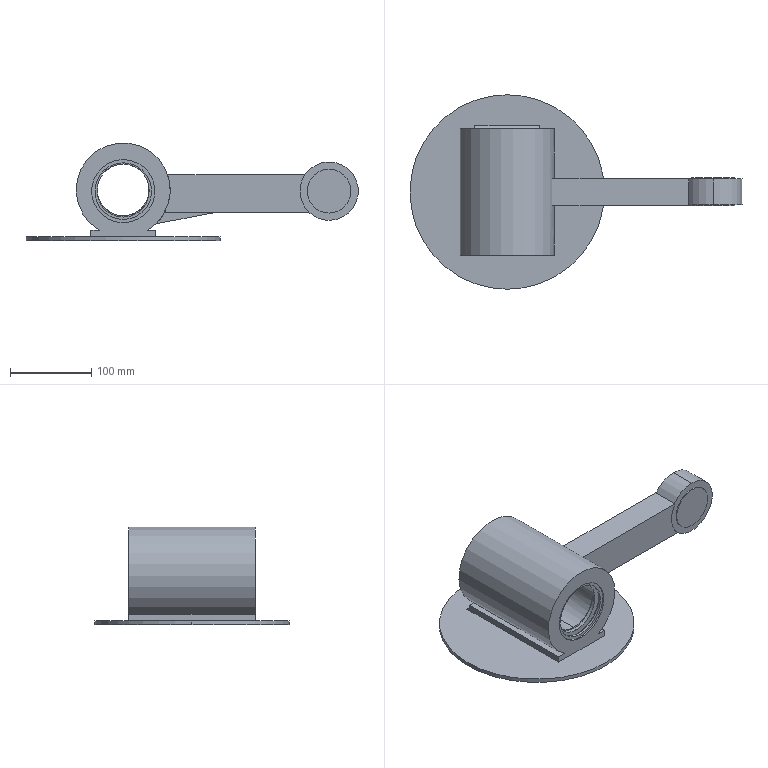Part | STEP file | Axle box 1 | 1 solid | 50 faces | box 410 x 240 x 120.8 mm | volume 1300329 mm3 | cylinder 25 | plane 25 | commonest cylinder face diameters 72 x5 54 x4 64 x4 70 x2 78 x2 78.4 x2
STEP:
#1=CARTESIAN_POINT('',(0.,-16.,-27.));
#2=VERTEX_POINT('',#1);
#3=CARTESIAN_POINT('',(0.,-16.,27.));
#4=VERTEX_POINT('',#3);
#5=CARTESIAN_POINT('',(0.,-16.,0.));
#6=DIRECTION('',(0.,-1.,0.));
#7=DIRECTION('',(0.,0.,1.));
#8=AXIS2_PLACEMENT_3D('',#5,#6,#7);
#9=CIRCLE('',#8,27.);
#10=EDGE_CURVE('',#2,#4,#9,.T.);
#11=ORIENTED_EDGE('',*,*,#10,.T.);
#12=CARTESIAN_POINT('',(0.,-17.2,27.));
#13=VERTEX_POINT('',#12);
#14=CARTESIAN_POINT('',(0.,17.2,27.));
#15=DIRECTION('',(0.,-1.,0.));
#16=VECTOR('',#15,1000.);
#17=LINE('',#14,#16);
#18=EDGE_CURVE('',#4,#13,#17,.T.);
#19=ORIENTED_EDGE('',*,*,#18,.T.);
#20=CARTESIAN_POINT('',(0.,-17.2,-27.));
#21=VERTEX_POINT('',#20);
#22=CARTESIAN_POINT('',(0.,-17.2,0.));
#23=DIRECTION('',(0.,1.,0.));
#24=DIRECTION('',(0.,0.,1.));
#25=AXIS2_PLACEMENT_3D('',#22,#23,#24);
#26=CIRCLE('',#25,27.);
#27=EDGE_CURVE('',#13,#21,#26,.T.);
#28=ORIENTED_EDGE('',*,*,#27,.T.);
#29=CARTESIAN_POINT('',(0.,17.2,-27.));
#30=DIRECTION('',(0.,-1.,0.));
#31=VECTOR('',#30,1000.);
#32=LINE('',#29,#31);
#33=EDGE_CURVE('',#2,#21,#32,.T.);
#34=ORIENTED_EDGE('',*,*,#33,.F.);
#35=EDGE_LOOP('',(#11,#19,#28,#34));
#36=FACE_OUTER_BOUND('',#35,.T.);
#37=CARTESIAN_POINT('',(0.,17.2,0.));
#38=DIRECTION('',(0.,-1.,0.));
#39=DIRECTION('',(0.,0.,-1.));
#40=AXIS2_PLACEMENT_3D('',#37,#38,#39);
#41=CYLINDRICAL_SURFACE('',#40,27.);
#42=ADVANCED_FACE('',(#36),#41,.T.);
#43=CARTESIAN_POINT('',(0.,17.2,27.));
#44=VERTEX_POINT('',#43);
#45=CARTESIAN_POINT('',(0.,17.2,-27.));
#46=VERTEX_POINT('',#45);
#47=CARTESIAN_POINT('',(0.,17.2,0.));
#48=DIRECTION('',(0.,1.,0.));
#49=DIRECTION('',(0.,0.,1.));
#50=AXIS2_PLACEMENT_3D('',#47,#48,#49);
#51=CIRCLE('',#50,27.);
#52=EDGE_CURVE('',#44,#46,#51,.T.);
#53=ORIENTED_EDGE('',*,*,#52,.F.);
#54=CARTESIAN_POINT('',(0.,16.,27.));
#55=VERTEX_POINT('',#54);
#56=CARTESIAN_POINT('',(0.,17.2,27.));
#57=DIRECTION('',(0.,-1.,0.));
#58=VECTOR('',#57,1000.);
#59=LINE('',#56,#58);
#60=EDGE_CURVE('',#44,#55,#59,.T.);
#61=ORIENTED_EDGE('',*,*,#60,.T.);
#62=CARTESIAN_POINT('',(0.,16.,-27.));
#63=VERTEX_POINT('',#62);
#64=CARTESIAN_POINT('',(0.,16.,0.));
#65=DIRECTION('',(0.,1.,0.));
#66=DIRECTION('',(0.,0.,1.));
#67=AXIS2_PLACEMENT_3D('',#64,#65,#66);
#68=CIRCLE('',#67,27.);
#69=EDGE_CURVE('',#55,#63,#68,.T.);
#70=ORIENTED_EDGE('',*,*,#69,.T.);
#71=CARTESIAN_POINT('',(0.,17.2,-27.));
#72=DIRECTION('',(0.,-1.,0.));
#73=VECTOR('',#72,1000.);
#74=LINE('',#71,#73);
#75=EDGE_CURVE('',#46,#63,#74,.T.);
#76=ORIENTED_EDGE('',*,*,#75,.F.);
#77=EDGE_LOOP('',(#53,#61,#70,#76));
#78=FACE_OUTER_BOUND('',#77,.T.);
#79=CARTESIAN_POINT('',(0.,17.2,0.));
#80=DIRECTION('',(0.,-1.,0.));
#81=DIRECTION('',(0.,0.,-1.));
#82=AXIS2_PLACEMENT_3D('',#79,#80,#81);
#83=CYLINDRICAL_SURFACE('',#82,27.);
#84=ADVANCED_FACE('',(#78),#83,.T.);
#85=CARTESIAN_POINT('',(-254.,-69.04,39.2));
#86=VERTEX_POINT('',#85);
#87=CARTESIAN_POINT('',(-254.,-69.04,-39.2));
#88=VERTEX_POINT('',#87);
#89=CARTESIAN_POINT('',(-254.,-69.04,0.));
#90=DIRECTION('',(0.,-1.,0.));
#91=DIRECTION('',(0.,0.,-1.));
#92=AXIS2_PLACEMENT_3D('',#89,#90,#91);
#93=CIRCLE('',#92,39.2);
#94=EDGE_CURVE('',#86,#88,#93,.T.);
#95=ORIENTED_EDGE('',*,*,#94,.F.);
#96=CARTESIAN_POINT('',(-254.,-73.04,39.2));
#97=VERTEX_POINT('',#96);
#98=CARTESIAN_POINT('',(-254.,-78.,39.2));
#99=DIRECTION('',(0.,-1.,0.));
#100=VECTOR('',#99,1000.);
#101=LINE('',#98,#100);
#102=EDGE_CURVE('',#86,#97,#101,.T.);
#103=ORIENTED_EDGE('',*,*,#102,.T.);
#104=CARTESIAN_POINT('',(-254.,-73.04,-39.2));
#105=VERTEX_POINT('',#104);
#106=CARTESIAN_POINT('',(-254.,-73.04,0.));
#107=DIRECTION('',(0.,-1.,0.));
#108=DIRECTION('',(0.,0.,-1.));
#109=AXIS2_PLACEMENT_3D('',#106,#107,#108);
#110=CIRCLE('',#109,39.2);
#111=EDGE_CURVE('',#97,#105,#110,.T.);
#112=ORIENTED_EDGE('',*,*,#111,.T.);
#113=CARTESIAN_POINT('',(-254.,-78.,-39.2));
#114=DIRECTION('',(0.,-1.,0.));
#115=VECTOR('',#114,1000.);
#116=LINE('',#113,#115);
#117=EDGE_CURVE('',#88,#105,#116,.T.);
#118=ORIENTED_EDGE('',*,*,#117,.F.);
#119=EDGE_LOOP('',(#95,#103,#112,#118));
#120=FACE_OUTER_BOUND('',#119,.T.);
#121=CARTESIAN_POINT('',(-254.,-78.,0.));
#122=DIRECTION('',(0.,-1.,0.));
#123=DIRECTION('',(0.,0.,-1.));
#124=AXIS2_PLACEMENT_3D('',#121,#122,#123);
#125=CYLINDRICAL_SURFACE('',#124,39.2);
#126=ADVANCED_FACE('',(#120),#125,.F.);
#127=CARTESIAN_POINT('',(-254.,-73.04,35.));
#128=VERTEX_POINT('',#127);
#129=CARTESIAN_POINT('',(-254.,-73.04,-35.));
#130=VERTEX_POINT('',#129);
#131=CARTESIAN_POINT('',(-254.,-73.04,0.));
#132=DIRECTION('',(0.,-1.,0.));
#133=DIRECTION('',(0.,0.,-1.));
#134=AXIS2_PLACEMENT_3D('',#131,#132,#133);
#135=CIRCLE('',#134,35.);
#136=EDGE_CURVE('',#128,#130,#135,.T.);
#137=ORIENTED_EDGE('',*,*,#136,.F.);
#138=CARTESIAN_POINT('',(-254.,-75.92,35.));
#139=VERTEX_POINT('',#138);
#140=CARTESIAN_POINT('',(-254.,-78.,35.));
#141=DIRECTION('',(0.,-1.,0.));
#142=VECTOR('',#141,1000.);
#143=LINE('',#140,#142);
#144=EDGE_CURVE('',#128,#139,#143,.T.);
#145=ORIENTED_EDGE('',*,*,#144,.T.);
#146=CARTESIAN_POINT('',(-254.,-75.92,-35.));
#147=VERTEX_POINT('',#146);
#148=CARTESIAN_POINT('',(-254.,-75.92,0.));
#149=DIRECTION('',(0.,-1.,0.));
#150=DIRECTION('',(0.,0.,-1.));
#151=AXIS2_PLACEMENT_3D('',#148,#149,#150);
#152=CIRCLE('',#151,35.);
#153=EDGE_CURVE('',#139,#147,#152,.T.);
#154=ORIENTED_EDGE('',*,*,#153,.T.);
#155=CARTESIAN_POINT('',(-254.,-78.,-35.));
#156=DIRECTION('',(0.,-1.,0.));
#157=VECTOR('',#156,1000.);
#158=LINE('',#155,#157);
#159=EDGE_CURVE('',#130,#147,#158,.T.);
#160=ORIENTED_EDGE('',*,*,#159,.F.);
#161=EDGE_LOOP('',(#137,#145,#154,#160));
#162=FACE_OUTER_BOUND('',#161,.T.);
#163=CARTESIAN_POINT('',(-254.,-78.,0.));
#164=DIRECTION('',(0.,-1.,0.));
#165=DIRECTION('',(0.,0.,-1.));
#166=AXIS2_PLACEMENT_3D('',#163,#164,#165);
#167=CYLINDRICAL_SURFACE('',#166,35.);
#168=ADVANCED_FACE('',(#162),#167,.F.);
#169=CARTESIAN_POINT('',(-254.,-75.92,39.));
#170=VERTEX_POINT('',#169);
#171=CARTESIAN_POINT('',(-254.,-75.92,-39.));
#172=VERTEX_POINT('',#171);
#173=CARTESIAN_POINT('',(-254.,-75.92,0.));
#174=DIRECTION('',(0.,-1.,0.));
#175=DIRECTION('',(0.,0.,-1.));
#176=AXIS2_PLACEMENT_3D('',#173,#174,#175);
#177=CIRCLE('',#176,39.);
#178=EDGE_CURVE('',#170,#172,#177,.T.);
#179=ORIENTED_EDGE('',*,*,#178,.F.);
#180=CARTESIAN_POINT('',(-254.,-78.,39.));
#181=VERTEX_POINT('',#180);
#182=CARTESIAN_POINT('',(-254.,-78.,39.));
#183=DIRECTION('',(0.,-1.,0.));
#184=VECTOR('',#183,1000.);
#185=LINE('',#182,#184);
#186=EDGE_CURVE('',#170,#181,#185,.T.);
#187=ORIENTED_EDGE('',*,*,#186,.T.);
#188=CARTESIAN_POINT('',(-254.,-78.,-39.));
#189=VERTEX_POINT('',#188);
#190=CARTESIAN_POINT('',(-254.,-78.,0.));
#191=DIRECTION('',(0.,-1.,0.));
#192=DIRECTION('',(0.,0.,-1.));
#193=AXIS2_PLACEMENT_3D('',#190,#191,#192);
#194=CIRCLE('',#193,39.);
#195=EDGE_CURVE('',#181,#189,#194,.T.);
#196=ORIENTED_EDGE('',*,*,#195,.T.);
#197=CARTESIAN_POINT('',(-254.,-78.,-39.));
#198=DIRECTION('',(0.,-1.,0.));
#199=VECTOR('',#198,1000.);
#200=LINE('',#197,#199);
#201=EDGE_CURVE('',#172,#189,#200,.T.);
#202=ORIENTED_EDGE('',*,*,#201,.F.);
#203=EDGE_LOOP('',(#179,#187,#196,#202));
#204=FACE_OUTER_BOUND('',#203,.T.);
#205=CARTESIAN_POINT('',(-254.,-78.,0.));
#206=DIRECTION('',(0.,-1.,0.));
#207=DIRECTION('',(0.,0.,-1.));
#208=AXIS2_PLACEMENT_3D('',#205,#206,#207);
#209=CYLINDRICAL_SURFACE('',#208,39.);
#210=ADVANCED_FACE('',(#204),#209,.F.);
#211=CARTESIAN_POINT('',(-254.,-64.8,-32.));
#212=VERTEX_POINT('',#211);
#213=CARTESIAN_POINT('',(-222.01,-64.8,0.8));
#214=VERTEX_POINT('',#213);
#215=CARTESIAN_POINT('',(-254.,-64.8,0.));
#216=DIRECTION('',(0.,-1.,0.));
#217=DIRECTION('',(0.,0.,-1.));
#218=AXIS2_PLACEMENT_3D('',#215,#216,#217);
#219=CIRCLE('',#218,32.);
#220=EDGE_CURVE('',#212,#214,#219,.T.);
#221=ORIENTED_EDGE('',*,*,#220,.F.);
#222=CARTESIAN_POINT('',(-254.,-69.04,-32.));
#223=VERTEX_POINT('',#222);
#224=CARTESIAN_POINT('',(-254.,-78.,-32.));
#225=DIRECTION('',(0.,-1.,0.));
#226=VECTOR('',#225,1000.);
#227=LINE('',#224,#226);
#228=EDGE_CURVE('',#212,#223,#227,.T.);
#229=ORIENTED_EDGE('',*,*,#228,.T.);
#230=CARTESIAN_POINT('',(-222.01,-69.04,0.8));
#231=VERTEX_POINT('',#230);
#232=CARTESIAN_POINT('',(-254.,-69.04,0.));
#233=DIRECTION('',(0.,-1.,0.));
#234=DIRECTION('',(0.,0.,-1.));
#235=AXIS2_PLACEMENT_3D('',#232,#233,#234);
#236=CIRCLE('',#235,32.);
#237=EDGE_CURVE('',#223,#231,#236,.T.);
#238=ORIENTED_EDGE('',*,*,#237,.T.);
#239=CARTESIAN_POINT('',(-222.01,-66.92,0.8));
#240=DIRECTION('',(0.,-1.,0.));
#241=VECTOR('',#240,1000.);
#242=LINE('',#239,#241);
#243=EDGE_CURVE('',#214,#231,#242,.T.);
#244=ORIENTED_EDGE('',*,*,#243,.F.);
#245=EDGE_LOOP('',(#221,#229,#238,#244));
#246=FACE_OUTER_BOUND('',#245,.T.);
#247=CARTESIAN_POINT('',(-254.,-78.,0.));
#248=DIRECTION('',(0.,-1.,0.));
#249=DIRECTION('',(0.,0.,-1.));
#250=AXIS2_PLACEMENT_3D('',#247,#248,#249);
#251=CYLINDRICAL_SURFACE('',#250,32.);
#252=ADVANCED_FACE('',(#246),#251,.F.);
#253=CARTESIAN_POINT('',(-374.,0.,-61.2));
#254=VERTEX_POINT('',#253);
#255=CARTESIAN_POINT('',(-134.,0.,-61.2));
#256=VERTEX_POINT('',#255);
#257=CARTESIAN_POINT('',(-254.,0.,-61.2));
#258=DIRECTION('',(0.,0.,-1.));
#259=DIRECTION('',(-1.,0.,0.));
#260=AXIS2_PLACEMENT_3D('',#257,#258,#259);
#261=CIRCLE('',#260,120.);
#262=EDGE_CURVE('',#254,#256,#261,.T.);
#263=ORIENTED_EDGE('',*,*,#262,.F.);
#264=CARTESIAN_POINT('',(-374.,0.,-56.4));
#265=VERTEX_POINT('',#264);
#266=CARTESIAN_POINT('',(-374.,0.,-61.2));
#267=DIRECTION('',(0.,0.,1.));
#268=VECTOR('',#267,1000.);
#269=LINE('',#266,#268);
#270=EDGE_CURVE('',#254,#265,#269,.T.);
#271=ORIENTED_EDGE('',*,*,#270,.T.);
#272=CARTESIAN_POINT('',(-134.,0.,-56.4));
#273=VERTEX_POINT('',#272);
#274=CARTESIAN_POINT('',(-254.,0.,-56.4));
#275=DIRECTION('',(0.,0.,-1.));
#276=DIRECTION('',(-1.,0.,0.));
#277=AXIS2_PLACEMENT_3D('',#274,#275,#276);
#278=CIRCLE('',#277,120.);
#279=EDGE_CURVE('',#265,#273,#278,.T.);
#280=ORIENTED_EDGE('',*,*,#279,.T.);
#281=CARTESIAN_POINT('',(-134.,0.,-61.2));
#282=DIRECTION('',(0.,0.,1.));
#283=VECTOR('',#282,1000.);
#284=LINE('',#281,#283);
#285=EDGE_CURVE('',#256,#273,#284,.T.);
#286=ORIENTED_EDGE('',*,*,#285,.F.);
#287=EDGE_LOOP('',(#263,#271,#280,#286));
#288=FACE_OUTER_BOUND('',#287,.T.);
#289=CARTESIAN_POINT('',(-254.,0.,-61.2));
#290=DIRECTION('',(0.,0.,1.));
#291=DIRECTION('',(1.,0.,0.));
#292=AXIS2_PLACEMENT_3D('',#289,#290,#291);
#293=CYLINDRICAL_SURFACE('',#292,120.);
#294=ADVANCED_FACE('',(#288),#293,.T.);
#295=CARTESIAN_POINT('',(-285.99,-64.8,0.8));
#296=VERTEX_POINT('',#295);
#297=CARTESIAN_POINT('',(-254.,-64.8,-30.4));
#298=VERTEX_POINT('',#297);
#299=CARTESIAN_POINT('',(-254.,-64.8,1.6));
#300=DIRECTION('',(0.,-1.,0.));
#301=DIRECTION('',(0.,0.,1.));
#302=AXIS2_PLACEMENT_3D('',#299,#300,#301);
#303=CIRCLE('',#302,32.);
#304=EDGE_CURVE('',#296,#298,#303,.T.);
#305=ORIENTED_EDGE('',*,*,#304,.T.);
#306=CARTESIAN_POINT('',(-254.,-22.,-30.4));
#307=VERTEX_POINT('',#306);
#308=CARTESIAN_POINT('',(-254.,-78.,-30.4));
#309=DIRECTION('',(0.,1.,0.));
#310=VECTOR('',#309,1000.);
#311=LINE('',#308,#310);
#312=EDGE_CURVE('',#298,#307,#311,.T.);
#313=ORIENTED_EDGE('',*,*,#312,.T.);
#314=CARTESIAN_POINT('',(-254.,-22.,33.6));
#315=VERTEX_POINT('',#314);
#316=CARTESIAN_POINT('',(-254.,-22.,1.6));
#317=DIRECTION('',(0.,1.,0.));
#318=DIRECTION('',(0.,0.,1.));
#319=AXIS2_PLACEMENT_3D('',#316,#317,#318);
#320=CIRCLE('',#319,32.);
#321=EDGE_CURVE('',#307,#315,#320,.T.);
#322=ORIENTED_EDGE('',*,*,#321,.T.);
#323=CARTESIAN_POINT('',(-254.,-69.04,33.6));
#324=VERTEX_POINT('',#323);
#325=CARTESIAN_POINT('',(-254.,-78.,33.6));
#326=DIRECTION('',(0.,1.,0.));
#327=VECTOR('',#326,1000.);
#328=LINE('',#325,#327);
#329=EDGE_CURVE('',#324,#315,#328,.T.);
#330=ORIENTED_EDGE('',*,*,#329,.F.);
#331=CARTESIAN_POINT('',(-285.99,-69.04,0.8));
#332=VERTEX_POINT('',#331);
#333=CARTESIAN_POINT('',(-254.,-69.04,1.6));
#334=DIRECTION('',(0.,-1.,0.));
#335=DIRECTION('',(0.,0.,1.));
#336=AXIS2_PLACEMENT_3D('',#333,#334,#335);
#337=CIRCLE('',#336,32.);
#338=EDGE_CURVE('',#324,#332,#337,.T.);
#339=ORIENTED_EDGE('',*,*,#338,.T.);
#340=CARTESIAN_POINT('',(-285.99,-66.92,0.8));
#341=DIRECTION('',(0.,1.,0.));
#342=VECTOR('',#341,1000.);
#343=LINE('',#340,#342);
#344=EDGE_CURVE('',#332,#296,#343,.T.);
#345=ORIENTED_EDGE('',*,*,#344,.T.);
#346=EDGE_LOOP('',(#305,#313,#322,#330,#339,#345));
#347=FACE_OUTER_BOUND('',#346,.T.);
#348=CARTESIAN_POINT('',(-254.,-78.,1.6));
#349=DIRECTION('',(0.,1.,0.));
#350=DIRECTION('',(0.,0.,1.));
#351=AXIS2_PLACEMENT_3D('',#348,#349,#350);
#352=CYLINDRICAL_SURFACE('',#351,32.);
#353=ADVANCED_FACE('',(#347),#352,.F.);
#354=CARTESIAN_POINT('',(-254.,-22.,52.6));
#355=VERTEX_POINT('',#354);
#356=CARTESIAN_POINT('',(-243.95,-22.,-48.4));
#357=VERTEX_POINT('',#356);
#358=CARTESIAN_POINT('',(-254.,-22.,1.6));
#359=DIRECTION('',(0.,1.,0.));
#360=DIRECTION('',(0.,0.,1.));
#361=AXIS2_PLACEMENT_3D('',#358,#359,#360);
#362=CIRCLE('',#361,51.);
#363=EDGE_CURVE('',#355,#357,#362,.T.);
#364=ORIENTED_EDGE('',*,*,#363,.F.);
#365=CARTESIAN_POINT('',(-254.,78.,52.6));
#366=VERTEX_POINT('',#365);
#367=CARTESIAN_POINT('',(-254.,-22.,52.6));
#368=DIRECTION('',(0.,1.,0.));
#369=VECTOR('',#368,1000.);
#370=LINE('',#367,#369);
#371=EDGE_CURVE('',#355,#366,#370,.T.);
#372=ORIENTED_EDGE('',*,*,#371,.T.);
#373=CARTESIAN_POINT('',(-243.95,78.,-48.4));
#374=VERTEX_POINT('',#373);
#375=CARTESIAN_POINT('',(-254.,78.,1.6));
#376=DIRECTION('',(0.,1.,0.));
#377=DIRECTION('',(0.,0.,1.));
#378=AXIS2_PLACEMENT_3D('',#375,#376,#377);
#379=CIRCLE('',#378,51.);
#380=EDGE_CURVE('',#366,#374,#379,.T.);
#381=ORIENTED_EDGE('',*,*,#380,.T.);
#382=CARTESIAN_POINT('',(-243.95,-22.,-48.4));
#383=DIRECTION('',(0.,-1.,0.));
#384=VECTOR('',#383,1000.);
#385=LINE('',#382,#384);
#386=EDGE_CURVE('',#374,#357,#385,.T.);
#387=ORIENTED_EDGE('',*,*,#386,.T.);
#388=EDGE_LOOP('',(#364,#372,#381,#387));
#389=FACE_OUTER_BOUND('',#388,.T.);
#390=CARTESIAN_POINT('',(-254.,-22.,1.6));
#391=DIRECTION('',(0.,1.,0.));
#392=DIRECTION('',(0.,0.,1.));
#393=AXIS2_PLACEMENT_3D('',#390,#391,#392);
#394=CYLINDRICAL_SURFACE('',#393,51.);
#395=ADVANCED_FACE('',(#389),#394,.F.);
#396=CARTESIAN_POINT('',(0.,-16.,36.));
#397=VERTEX_POINT('',#396);
#398=CARTESIAN_POINT('',(0.,-16.,-36.));
#399=VERTEX_POINT('',#398);
#400=CARTESIAN_POINT('',(0.,-16.,0.));
#401=DIRECTION('',(0.,1.,0.));
#402=DIRECTION('',(0.,0.,1.));
#403=AXIS2_PLACEMENT_3D('',#400,#401,#402);
#404=CIRCLE('',#403,36.);
#405=EDGE_CURVE('',#397,#399,#404,.T.);
#406=ORIENTED_EDGE('',*,*,#405,.T.);
#407=CARTESIAN_POINT('',(0.,16.,-36.));
#408=VERTEX_POINT('',#407);
#409=CARTESIAN_POINT('',(0.,-16.,-36.));
#410=DIRECTION('',(0.,1.,0.));
#411=VECTOR('',#410,1000.);
#412=LINE('',#409,#411);
#413=EDGE_CURVE('',#399,#408,#412,.T.);
#414=ORIENTED_EDGE('',*,*,#413,.T.);
#415=CARTESIAN_POINT('',(0.,16.,36.));
#416=VERTEX_POINT('',#415);
#417=CARTESIAN_POINT('',(0.,16.,0.));
#418=DIRECTION('',(0.,1.,0.));
#419=DIRECTION('',(0.,0.,1.));
#420=AXIS2_PLACEMENT_3D('',#417,#418,#419);
#421=CIRCLE('',#420,36.);
#422=EDGE_CURVE('',#416,#408,#421,.T.);
#423=ORIENTED_EDGE('',*,*,#422,.F.);
#424=CARTESIAN_POINT('',(0.,-16.,36.));
#425=DIRECTION('',(0.,1.,0.));
#426=VECTOR('',#425,1000.);
#427=LINE('',#424,#426);
#428=EDGE_CURVE('',#397,#416,#427,.T.);
#429=ORIENTED_EDGE('',*,*,#428,.F.);
#430=EDGE_LOOP('',(#406,#414,#423,#429));
#431=FACE_OUTER_BOUND('',#430,.T.);
#432=CARTESIAN_POINT('',(0.,-16.,0.));
#433=DIRECTION('',(0.,1.,0.));
#434=DIRECTION('',(0.,0.,1.));
#435=AXIS2_PLACEMENT_3D('',#432,#433,#434);
#436=CYLINDRICAL_SURFACE('',#435,36.);
#437=ADVANCED_FACE('',(#431),#436,.T.);
#438=CARTESIAN_POINT('',(-29.933,-16.,20.));
#439=VERTEX_POINT('',#438);
#440=CARTESIAN_POINT('',(0.,-16.,0.));
#441=DIRECTION('',(0.,1.,0.));
#442=DIRECTION('',(0.,0.,1.));
#443=AXIS2_PLACEMENT_3D('',#440,#441,#442);
#444=CIRCLE('',#443,36.);
#445=EDGE_CURVE('',#439,#397,#444,.T.);
#446=ORIENTED_EDGE('',*,*,#445,.T.);
#447=ORIENTED_EDGE('',*,*,#428,.T.);
#448=CARTESIAN_POINT('',(-29.933,16.,20.));
#449=VERTEX_POINT('',#448);
#450=CARTESIAN_POINT('',(0.,16.,0.));
#451=DIRECTION('',(0.,1.,0.));
#452=DIRECTION('',(0.,0.,1.));
#453=AXIS2_PLACEMENT_3D('',#450,#451,#452);
#454=CIRCLE('',#453,36.);
#455=EDGE_CURVE('',#449,#416,#454,.T.);
#456=ORIENTED_EDGE('',*,*,#455,.F.);
#457=CARTESIAN_POINT('',(-29.933,-16.8,20.));
#458=DIRECTION('',(0.,1.,0.));
#459=VECTOR('',#458,1000.);
#460=LINE('',#457,#459);
#461=EDGE_CURVE('',#439,#449,#460,.T.);
#462=ORIENTED_EDGE('',*,*,#461,.F.);
#463=EDGE_LOOP('',(#446,#447,#456,#462));
#464=FACE_OUTER_BOUND('',#463,.T.);
#465=CARTESIAN_POINT('',(0.,-16.,0.));
#466=DIRECTION('',(0.,1.,0.));
#467=DIRECTION('',(0.,0.,1.));
#468=AXIS2_PLACEMENT_3D('',#465,#466,#467);
#469=CYLINDRICAL_SURFACE('',#468,36.);
#470=ADVANCED_FACE('',(#464),#469,.T.);
#471=ORIENTED_EDGE('',*,*,#413,.F.);
#472=CARTESIAN_POINT('',(-24.9,-16.,-26.));
#473=VERTEX_POINT('',#472);
#474=CARTESIAN_POINT('',(0.,-16.,0.));
#475=DIRECTION('',(0.,1.,0.));
#476=DIRECTION('',(0.,0.,1.));
#477=AXIS2_PLACEMENT_3D('',#474,#475,#476);
#478=CIRCLE('',#477,36.);
#479=EDGE_CURVE('',#399,#473,#478,.T.);
#480=ORIENTED_EDGE('',*,*,#479,.T.);
#481=CARTESIAN_POINT('',(-24.9,16.,-26.));
#482=VERTEX_POINT('',#481);
#483=CARTESIAN_POINT('',(-24.9,-16.8,-26.));
#484=DIRECTION('',(0.,1.,0.));
#485=VECTOR('',#484,1000.);
#486=LINE('',#483,#485);
#487=EDGE_CURVE('',#473,#482,#486,.T.);
#488=ORIENTED_EDGE('',*,*,#487,.T.);
#489=CARTESIAN_POINT('',(0.,16.,0.));
#490=DIRECTION('',(0.,1.,0.));
#491=DIRECTION('',(0.,0.,1.));
#492=AXIS2_PLACEMENT_3D('',#489,#490,#491);
#493=CIRCLE('',#492,36.);
#494=EDGE_CURVE('',#408,#482,#493,.T.);
#495=ORIENTED_EDGE('',*,*,#494,.F.);
#496=EDGE_LOOP('',(#471,#480,#488,#495));
#497=FACE_OUTER_BOUND('',#496,.T.);
#498=CARTESIAN_POINT('',(0.,-16.,0.));
#499=DIRECTION('',(0.,1.,0.));
#500=DIRECTION('',(0.,0.,1.));
#501=AXIS2_PLACEMENT_3D('',#498,#499,#500);
#502=CYLINDRICAL_SURFACE('',#501,36.);
#503=ADVANCED_FACE('',(#497),#502,.T.);
#504=ORIENTED_EDGE('',*,*,#10,.F.);
#505=CARTESIAN_POINT('',(0.,-16.,0.));
#506=DIRECTION('',(0.,-1.,0.));
#507=DIRECTION('',(0.,0.,1.));
#508=AXIS2_PLACEMENT_3D('',#505,#506,#507);
#509=CIRCLE('',#508,27.);
#510=EDGE_CURVE('',#4,#2,#509,.T.);
#511=ORIENTED_EDGE('',*,*,#510,.F.);
#512=EDGE_LOOP('',(#504,#511));
#513=FACE_BOUND('',#512,.T.);
#514=CARTESIAN_POINT('',(0.,-16.,0.));
#515=DIRECTION('',(0.,1.,0.));
#516=DIRECTION('',(0.,0.,1.));
#517=AXIS2_PLACEMENT_3D('',#514,#515,#516);
#518=CIRCLE('',#517,36.);
#519=EDGE_CURVE('',#473,#439,#518,.T.);
#520=ORIENTED_EDGE('',*,*,#519,.F.);
#521=ORIENTED_EDGE('',*,*,#479,.F.);
#522=ORIENTED_EDGE('',*,*,#405,.F.);
#523=ORIENTED_EDGE('',*,*,#445,.F.);
#524=EDGE_LOOP('',(#520,#521,#522,#523));
#525=FACE_OUTER_BOUND('',#524,.T.);
#526=CARTESIAN_POINT('',(0.,-16.,0.));
#527=DIRECTION('',(0.,1.,0.));
#528=DIRECTION('',(0.,0.,1.));
#529=AXIS2_PLACEMENT_3D('',#526,#527,#528);
#530=PLANE('',#529);
#531=ADVANCED_FACE('',(#513,#525),#530,.F.);
#532=CARTESIAN_POINT('',(0.,16.,0.));
#533=DIRECTION('',(0.,1.,0.));
#534=DIRECTION('',(0.,0.,1.));
#535=AXIS2_PLACEMENT_3D('',#532,#533,#534);
#536=CIRCLE('',#535,27.);
#537=EDGE_CURVE('',#63,#55,#536,.T.);
#538=ORIENTED_EDGE('',*,*,#537,.F.);
#539=ORIENTED_EDGE('',*,*,#69,.F.);
#540=EDGE_LOOP('',(#538,#539));
#541=FACE_BOUND('',#540,.T.);
#542=CARTESIAN_POINT('',(0.,16.,0.));
#543=DIRECTION('',(0.,1.,0.));
#544=DIRECTION('',(0.,0.,1.));
#545=AXIS2_PLACEMENT_3D('',#542,#543,#544);
#546=CIRCLE('',#545,36.);
#547=EDGE_CURVE('',#482,#449,#546,.T.);
#548=ORIENTED_EDGE('',*,*,#547,.T.);
#549=ORIENTED_EDGE('',*,*,#455,.T.);
#550=ORIENTED_EDGE('',*,*,#422,.T.);
#551=ORIENTED_EDGE('',*,*,#494,.T.);
#552=EDGE_LOOP('',(#548,#549,#550,#551));
#553=FACE_OUTER_BOUND('',#552,.T.);
#554=CARTESIAN_POINT('',(0.,16.,0.));
#555=DIRECTION('',(0.,1.,0.));
#556=DIRECTION('',(0.,0.,1.));
#557=AXIS2_PLACEMENT_3D('',#554,#555,#556);
#558=PLANE('',#557);
#559=ADVANCED_FACE('',(#541,#553),#558,.T.);
#560=CARTESIAN_POINT('',(-24.9,-16.8,-26.));
#561=VERTEX_POINT('',#560);
#562=CARTESIAN_POINT('',(-24.9,-16.8,-26.));
#563=DIRECTION('',(0.,1.,0.));
#564=VECTOR('',#563,1000.);
#565=LINE('',#562,#564);
#566=EDGE_CURVE('',#561,#473,#565,.T.);
#567=ORIENTED_EDGE('',*,*,#566,.T.);
#568=ORIENTED_EDGE('',*,*,#519,.T.);
#569=CARTESIAN_POINT('',(-29.933,-16.8,20.));
#570=VERTEX_POINT('',#569);
#571=CARTESIAN_POINT('',(-29.933,-16.8,20.));
#572=DIRECTION('',(0.,1.,0.));
#573=VECTOR('',#572,1000.);
#574=LINE('',#571,#573);
#575=EDGE_CURVE('',#570,#439,#574,.T.);
#576=ORIENTED_EDGE('',*,*,#575,.F.);
#577=CARTESIAN_POINT('',(0.,-16.8,0.));
#578=DIRECTION('',(0.,1.,0.));
#579=DIRECTION('',(0.,0.,1.));
#580=AXIS2_PLACEMENT_3D('',#577,#578,#579);
#581=CIRCLE('',#580,36.);
#582=EDGE_CURVE('',#561,#570,#581,.T.);
#583=ORIENTED_EDGE('',*,*,#582,.F.);
#584=EDGE_LOOP('',(#567,#568,#576,#583));
#585=FACE_OUTER_BOUND('',#584,.T.);
#586=CARTESIAN_POINT('',(0.,-16.8,0.));
#587=DIRECTION('',(0.,1.,0.));
#588=DIRECTION('',(0.,0.,1.));
#589=AXIS2_PLACEMENT_3D('',#586,#587,#588);
#590=CYLINDRICAL_SURFACE('',#589,36.);
#591=ADVANCED_FACE('',(#585),#590,.F.);
#592=ORIENTED_EDGE('',*,*,#547,.F.);
#593=CARTESIAN_POINT('',(-24.9,16.8,-26.));
#594=VERTEX_POINT('',#593);
#595=CARTESIAN_POINT('',(-24.9,-16.8,-26.));
#596=DIRECTION('',(0.,1.,0.));
#597=VECTOR('',#596,1000.);
#598=LINE('',#595,#597);
#599=EDGE_CURVE('',#482,#594,#598,.T.);
#600=ORIENTED_EDGE('',*,*,#599,.T.);
#601=CARTESIAN_POINT('',(-29.933,16.8,20.));
#602=VERTEX_POINT('',#601);
#603=CARTESIAN_POINT('',(0.,16.8,0.));
#604=DIRECTION('',(0.,1.,0.));
#605=DIRECTION('',(0.,0.,1.));
#606=AXIS2_PLACEMENT_3D('',#603,#604,#605);
#607=CIRCLE('',#606,36.);
#608=EDGE_CURVE('',#594,#602,#607,.T.);
#609=ORIENTED_EDGE('',*,*,#608,.T.);
#610=CARTESIAN_POINT('',(-29.933,-16.8,20.));
#611=DIRECTION('',(0.,1.,0.));
#612=VECTOR('',#611,1000.);
#613=LINE('',#610,#612);
#614=EDGE_CURVE('',#449,#602,#613,.T.);
#615=ORIENTED_EDGE('',*,*,#614,.F.);
#616=EDGE_LOOP('',(#592,#600,#609,#615));
#617=FACE_OUTER_BOUND('',#616,.T.);
#618=CARTESIAN_POINT('',(0.,-16.8,0.));
#619=DIRECTION('',(0.,1.,0.));
#620=DIRECTION('',(0.,0.,1.));
#621=AXIS2_PLACEMENT_3D('',#618,#619,#620);
#622=CYLINDRICAL_SURFACE('',#621,36.);
#623=ADVANCED_FACE('',(#617),#622,.F.);
#624=ORIENTED_EDGE('',*,*,#575,.T.);
#625=ORIENTED_EDGE('',*,*,#461,.T.);
#626=ORIENTED_EDGE('',*,*,#614,.T.);
#627=CARTESIAN_POINT('',(-198.996,16.8,20.));
#628=VERTEX_POINT('',#627);
#629=CARTESIAN_POINT('',(0.,16.8,20.));
#630=DIRECTION('',(1.,0.,0.));
#631=VECTOR('',#630,1000.);
#632=LINE('',#629,#631);
#633=EDGE_CURVE('',#628,#602,#632,.T.);
#634=ORIENTED_EDGE('',*,*,#633,.F.);
#635=CARTESIAN_POINT('',(-198.996,-16.8,20.));
#636=VERTEX_POINT('',#635);
#637=CARTESIAN_POINT('',(-198.996,-16.8,20.));
#638=DIRECTION('',(0.,1.,0.));
#639=VECTOR('',#638,1000.);
#640=LINE('',#637,#639);
#641=EDGE_CURVE('',#636,#628,#640,.T.);
#642=ORIENTED_EDGE('',*,*,#641,.F.);
#643=CARTESIAN_POINT('',(0.,-16.8,20.));
#644=DIRECTION('',(1.,0.,0.));
#645=VECTOR('',#644,1000.);
#646=LINE('',#643,#645);
#647=EDGE_CURVE('',#636,#570,#646,.T.);
#648=ORIENTED_EDGE('',*,*,#647,.T.);
#649=EDGE_LOOP('',(#624,#625,#626,#634,#642,#648));
#650=FACE_OUTER_BOUND('',#649,.T.);
#651=CARTESIAN_POINT('',(0.,-16.8,20.));
#652=DIRECTION('',(0.,0.,1.));
#653=DIRECTION('',(1.,0.,0.));
#654=AXIS2_PLACEMENT_3D('',#651,#652,#653);
#655=PLANE('',#654);
#656=ADVANCED_FACE('',(#650),#655,.T.);
#657=CARTESIAN_POINT('',(-138.988,2.,-26.));
#658=VERTEX_POINT('',#657);
#659=CARTESIAN_POINT('',(-138.988,-2.,-26.));
#660=VERTEX_POINT('',#659);
#661=CARTESIAN_POINT('',(-138.988,2.,-26.));
#662=DIRECTION('',(0.,-1.,0.));
#663=VECTOR('',#662,1000.);
#664=LINE('',#661,#663);
#665=EDGE_CURVE('',#658,#660,#664,.T.);
#666=ORIENTED_EDGE('',*,*,#665,.F.);
#667=CARTESIAN_POINT('',(-202.988,2.,-26.));
#668=VERTEX_POINT('',#667);
#669=CARTESIAN_POINT('',(0.,2.,-26.));
#670=DIRECTION('',(1.,0.,0.));
#671=VECTOR('',#670,1000.);
#672=LINE('',#669,#671);
#673=EDGE_CURVE('',#668,#658,#672,.T.);
#674=ORIENTED_EDGE('',*,*,#673,.F.);
#675=CARTESIAN_POINT('',(-202.988,16.8,-26.));
#676=VERTEX_POINT('',#675);
#677=CARTESIAN_POINT('',(-202.988,-16.8,-26.));
#678=DIRECTION('',(0.,1.,0.));
#679=VECTOR('',#678,1000.);
#680=LINE('',#677,#679);
#681=EDGE_CURVE('',#668,#676,#680,.T.);
#682=ORIENTED_EDGE('',*,*,#681,.T.);
#683=CARTESIAN_POINT('',(0.,16.8,-26.));
#684=DIRECTION('',(1.,0.,0.));
#685=VECTOR('',#684,1000.);
#686=LINE('',#683,#685);
#687=EDGE_CURVE('',#676,#594,#686,.T.);
#688=ORIENTED_EDGE('',*,*,#687,.T.);
#689=ORIENTED_EDGE('',*,*,#599,.F.);
#690=ORIENTED_EDGE('',*,*,#487,.F.);
#691=ORIENTED_EDGE('',*,*,#566,.F.);
#692=CARTESIAN_POINT('',(-202.988,-16.8,-26.));
#693=VERTEX_POINT('',#692);
#694=CARTESIAN_POINT('',(0.,-16.8,-26.));
#695=DIRECTION('',(1.,0.,0.));
#696=VECTOR('',#695,1000.);
#697=LINE('',#694,#696);
#698=EDGE_CURVE('',#693,#561,#697,.T.);
#699=ORIENTED_EDGE('',*,*,#698,.F.);
#700=CARTESIAN_POINT('',(-202.988,-2.,-26.));
#701=VERTEX_POINT('',#700);
#702=CARTESIAN_POINT('',(-202.988,-16.8,-26.));
#703=DIRECTION('',(0.,1.,0.));
#704=VECTOR('',#703,1000.);
#705=LINE('',#702,#704);
#706=EDGE_CURVE('',#693,#701,#705,.T.);
#707=ORIENTED_EDGE('',*,*,#706,.T.);
#708=CARTESIAN_POINT('',(0.,-2.,-26.));
#709=DIRECTION('',(1.,0.,0.));
#710=VECTOR('',#709,1000.);
#711=LINE('',#708,#710);
#712=EDGE_CURVE('',#701,#660,#711,.T.);
#713=ORIENTED_EDGE('',*,*,#712,.T.);
#714=EDGE_LOOP('',(#666,#674,#682,#688,#689,#690,#691,#699,#707,#713));
#715=FACE_OUTER_BOUND('',#714,.T.);
#716=CARTESIAN_POINT('',(0.,-16.8,-26.));
#717=DIRECTION('',(0.,0.,1.));
#718=DIRECTION('',(1.,0.,0.));
#719=AXIS2_PLACEMENT_3D('',#716,#717,#718);
#720=PLANE('',#719);
#721=ADVANCED_FACE('',(#715),#720,.F.);
#722=ORIENTED_EDGE('',*,*,#582,.T.);
#723=ORIENTED_EDGE('',*,*,#647,.F.);
#724=CARTESIAN_POINT('',(-254.,-16.8,1.6));
#725=DIRECTION('',(0.,1.,0.));
#726=DIRECTION('',(0.,0.,1.));
#727=AXIS2_PLACEMENT_3D('',#724,#725,#726);
#728=CIRCLE('',#727,58.);
#729=EDGE_CURVE('',#636,#693,#728,.T.);
#730=ORIENTED_EDGE('',*,*,#729,.T.);
#731=ORIENTED_EDGE('',*,*,#698,.T.);
#732=EDGE_LOOP('',(#722,#723,#730,#731));
#733=FACE_OUTER_BOUND('',#732,.T.);
#734=CARTESIAN_POINT('',(0.,-16.8,0.));
#735=DIRECTION('',(0.,1.,0.));
#736=DIRECTION('',(0.,0.,1.));
#737=AXIS2_PLACEMENT_3D('',#734,#735,#736);
#738=PLANE('',#737);
#739=ADVANCED_FACE('',(#733),#738,.F.);
#740=ORIENTED_EDGE('',*,*,#608,.F.);
#741=ORIENTED_EDGE('',*,*,#687,.F.);
#742=CARTESIAN_POINT('',(-254.,16.8,1.6));
#743=DIRECTION('',(0.,1.,0.));
#744=DIRECTION('',(0.,0.,1.));
#745=AXIS2_PLACEMENT_3D('',#742,#743,#744);
#746=CIRCLE('',#745,58.);
#747=EDGE_CURVE('',#628,#676,#746,.T.);
#748=ORIENTED_EDGE('',*,*,#747,.F.);
#749=ORIENTED_EDGE('',*,*,#633,.T.);
#750=EDGE_LOOP('',(#740,#741,#748,#749));
#751=FACE_OUTER_BOUND('',#750,.T.);
#752=CARTESIAN_POINT('',(0.,16.8,0.));
#753=DIRECTION('',(0.,1.,0.));
#754=DIRECTION('',(0.,0.,1.));
#755=AXIS2_PLACEMENT_3D('',#752,#753,#754);
#756=PLANE('',#755);
#757=ADVANCED_FACE('',(#751),#756,.T.);
#758=CARTESIAN_POINT('',(-283.394,78.,-48.4));
#759=VERTEX_POINT('',#758);
#760=CARTESIAN_POINT('',(-224.606,78.,-48.4));
#761=VERTEX_POINT('',#760);
#762=CARTESIAN_POINT('',(-254.,78.,1.6));
#763=DIRECTION('',(0.,1.,0.));
#764=DIRECTION('',(0.,0.,1.));
#765=AXIS2_PLACEMENT_3D('',#762,#763,#764);
#766=CIRCLE('',#765,58.);
#767=EDGE_CURVE('',#759,#761,#766,.T.);
#768=ORIENTED_EDGE('',*,*,#767,.F.);
#769=CARTESIAN_POINT('',(-283.394,-78.,-48.4));
#770=VERTEX_POINT('',#769);
#771=CARTESIAN_POINT('',(-283.394,78.,-48.4));
#772=DIRECTION('',(0.,-1.,0.));
#773=VECTOR('',#772,1000.);
#774=LINE('',#771,#773);
#775=EDGE_CURVE('',#759,#770,#774,.T.);
#776=ORIENTED_EDGE('',*,*,#775,.T.);
#777=CARTESIAN_POINT('',(-224.606,-78.,-48.4));
#778=VERTEX_POINT('',#777);
#779=CARTESIAN_POINT('',(-254.,-78.,1.6));
#780=DIRECTION('',(0.,1.,0.));
#781=DIRECTION('',(0.,0.,1.));
#782=AXIS2_PLACEMENT_3D('',#779,#780,#781);
#783=CIRCLE('',#782,58.);
#784=EDGE_CURVE('',#770,#778,#783,.T.);
#785=ORIENTED_EDGE('',*,*,#784,.T.);
#786=CARTESIAN_POINT('',(-224.606,78.,-48.4));
#787=DIRECTION('',(0.,1.,0.));
#788=VECTOR('',#787,1000.);
#789=LINE('',#786,#788);
#790=EDGE_CURVE('',#778,#761,#789,.T.);
#791=ORIENTED_EDGE('',*,*,#790,.T.);
#792=EDGE_LOOP('',(#768,#776,#785,#791));
#793=FACE_OUTER_BOUND('',#792,.T.);
#794=ORIENTED_EDGE('',*,*,#681,.F.);
#795=CARTESIAN_POINT('',(-214.,2.,-40.4));
#796=VERTEX_POINT('',#795);
#797=CARTESIAN_POINT('',(-254.,2.,1.6));
#798=DIRECTION('',(0.,1.,0.));
#799=DIRECTION('',(0.,0.,1.));
#800=AXIS2_PLACEMENT_3D('',#797,#798,#799);
#801=CIRCLE('',#800,58.);
#802=EDGE_CURVE('',#668,#796,#801,.T.);
#803=ORIENTED_EDGE('',*,*,#802,.T.);
#804=CARTESIAN_POINT('',(-214.,-2.,-40.4));
#805=VERTEX_POINT('',#804);
#806=CARTESIAN_POINT('',(-214.,2.,-40.4));
#807=DIRECTION('',(0.,-1.,0.));
#808=VECTOR('',#807,1000.);
#809=LINE('',#806,#808);
#810=EDGE_CURVE('',#796,#805,#809,.T.);
#811=ORIENTED_EDGE('',*,*,#810,.T.);
#812=CARTESIAN_POINT('',(-254.,-2.,1.6));
#813=DIRECTION('',(0.,1.,0.));
#814=DIRECTION('',(0.,0.,1.));
#815=AXIS2_PLACEMENT_3D('',#812,#813,#814);
#816=CIRCLE('',#815,58.);
#817=EDGE_CURVE('',#701,#805,#816,.T.);
#818=ORIENTED_EDGE('',*,*,#817,.F.);
#819=ORIENTED_EDGE('',*,*,#706,.F.);
#820=ORIENTED_EDGE('',*,*,#729,.F.);
#821=ORIENTED_EDGE('',*,*,#641,.T.);
#822=ORIENTED_EDGE('',*,*,#747,.T.);
#823=EDGE_LOOP('',(#794,#803,#811,#818,#819,#820,#821,#822));
#824=FACE_BOUND('',#823,.T.);
#825=CARTESIAN_POINT('',(-254.,78.,1.6));
#826=DIRECTION('',(0.,-1.,0.));
#827=DIRECTION('',(0.,0.,-1.));
#828=AXIS2_PLACEMENT_3D('',#825,#826,#827);
#829=CYLINDRICAL_SURFACE('',#828,58.);
#830=ADVANCED_FACE('',(#793,#824),#829,.T.);
#831=CARTESIAN_POINT('',(-264.05,78.,-48.4));
#832=VERTEX_POINT('',#831);
#833=CARTESIAN_POINT('',(-254.,78.,1.6));
#834=DIRECTION('',(0.,1.,0.));
#835=DIRECTION('',(0.,0.,1.));
#836=AXIS2_PLACEMENT_3D('',#833,#834,#835);
#837=CIRCLE('',#836,51.);
#838=EDGE_CURVE('',#832,#366,#837,.T.);
#839=ORIENTED_EDGE('',*,*,#838,.F.);
#840=CARTESIAN_POINT('',(-294.,78.,-48.4));
#841=DIRECTION('',(1.,0.,0.));
#842=VECTOR('',#841,1000.);
#843=LINE('',#840,#842);
#844=EDGE_CURVE('',#832,#374,#843,.T.);
#845=ORIENTED_EDGE('',*,*,#844,.T.);
#846=ORIENTED_EDGE('',*,*,#380,.F.);
#847=EDGE_LOOP('',(#839,#845,#846));
#848=FACE_BOUND('',#847,.T.);
#849=CARTESIAN_POINT('',(-214.,78.,-48.4));
#850=VERTEX_POINT('',#849);
#851=CARTESIAN_POINT('',(-214.,78.,-52.4));
#852=VERTEX_POINT('',#851);
#853=CARTESIAN_POINT('',(-214.,78.,-56.4));
#854=DIRECTION('',(0.,0.,-1.));
#855=VECTOR('',#854,1000.);
#856=LINE('',#853,#855);
#857=EDGE_CURVE('',#850,#852,#856,.T.);
#858=ORIENTED_EDGE('',*,*,#857,.T.);
#859=CARTESIAN_POINT('',(-294.,78.,-52.4));
#860=VERTEX_POINT('',#859);
#861=CARTESIAN_POINT('',(-254.,78.,-52.4));
#862=DIRECTION('',(-1.,0.,0.));
#863=VECTOR('',#862,1000.);
#864=LINE('',#861,#863);
#865=EDGE_CURVE('',#852,#860,#864,.T.);
#866=ORIENTED_EDGE('',*,*,#865,.T.);
#867=CARTESIAN_POINT('',(-294.,78.,-48.4));
#868=VERTEX_POINT('',#867);
#869=CARTESIAN_POINT('',(-294.,78.,-56.4));
#870=DIRECTION('',(0.,0.,1.));
#871=VECTOR('',#870,1000.);
#872=LINE('',#869,#871);
#873=EDGE_CURVE('',#860,#868,#872,.T.);
#874=ORIENTED_EDGE('',*,*,#873,.T.);
#875=CARTESIAN_POINT('',(-294.,78.,-48.4));
#876=DIRECTION('',(1.,0.,0.));
#877=VECTOR('',#876,1000.);
#878=LINE('',#875,#877);
#879=EDGE_CURVE('',#868,#759,#878,.T.);
#880=ORIENTED_EDGE('',*,*,#879,.T.);
#881=ORIENTED_EDGE('',*,*,#767,.T.);
#882=CARTESIAN_POINT('',(-294.,78.,-48.4));
#883=DIRECTION('',(1.,0.,0.));
#884=VECTOR('',#883,1000.);
#885=LINE('',#882,#884);
#886=EDGE_CURVE('',#761,#850,#885,.T.);
#887=ORIENTED_EDGE('',*,*,#886,.T.);
#888=EDGE_LOOP('',(#858,#866,#874,#880,#881,#887));
#889=FACE_OUTER_BOUND('',#888,.T.);
#890=CARTESIAN_POINT('',(-254.,78.,1.6));
#891=DIRECTION('',(0.,1.,0.));
#892=DIRECTION('',(0.,0.,1.));
#893=AXIS2_PLACEMENT_3D('',#890,#891,#892);
#894=PLANE('',#893);
#895=ADVANCED_FACE('',(#848,#889),#894,.T.);
#896=CARTESIAN_POINT('',(-254.,-78.,0.));
#897=DIRECTION('',(0.,-1.,0.));
#898=DIRECTION('',(0.,0.,-1.));
#899=AXIS2_PLACEMENT_3D('',#896,#897,#898);
#900=CIRCLE('',#899,39.);
#901=EDGE_CURVE('',#189,#181,#900,.T.);
#902=ORIENTED_EDGE('',*,*,#901,.F.);
#903=ORIENTED_EDGE('',*,*,#195,.F.);
#904=EDGE_LOOP('',(#902,#903));
#905=FACE_BOUND('',#904,.T.);
#906=ORIENTED_EDGE('',*,*,#784,.F.);
#907=CARTESIAN_POINT('',(-294.,-78.,-48.4));
#908=VERTEX_POINT('',#907);
#909=CARTESIAN_POINT('',(-294.,-78.,-48.4));
#910=DIRECTION('',(1.,0.,0.));
#911=VECTOR('',#910,1000.);
#912=LINE('',#909,#911);
#913=EDGE_CURVE('',#908,#770,#912,.T.);
#914=ORIENTED_EDGE('',*,*,#913,.F.);
#915=CARTESIAN_POINT('',(-294.,-78.,-56.4));
#916=VERTEX_POINT('',#915);
#917=CARTESIAN_POINT('',(-294.,-78.,-56.4));
#918=DIRECTION('',(0.,0.,1.));
#919=VECTOR('',#918,1000.);
#920=LINE('',#917,#919);
#921=EDGE_CURVE('',#916,#908,#920,.T.);
#922=ORIENTED_EDGE('',*,*,#921,.F.);
#923=CARTESIAN_POINT('',(-214.,-78.,-56.4));
#924=VERTEX_POINT('',#923);
#925=CARTESIAN_POINT('',(-294.,-78.,-56.4));
#926=DIRECTION('',(-1.,0.,0.));
#927=VECTOR('',#926,1000.);
#928=LINE('',#925,#927);
#929=EDGE_CURVE('',#924,#916,#928,.T.);
#930=ORIENTED_EDGE('',*,*,#929,.F.);
#931=CARTESIAN_POINT('',(-214.,-78.,-48.4));
#932=VERTEX_POINT('',#931);
#933=CARTESIAN_POINT('',(-214.,-78.,-56.4));
#934=DIRECTION('',(0.,0.,-1.));
#935=VECTOR('',#934,1000.);
#936=LINE('',#933,#935);
#937=EDGE_CURVE('',#932,#924,#936,.T.);
#938=ORIENTED_EDGE('',*,*,#937,.F.);
#939=CARTESIAN_POINT('',(-294.,-78.,-48.4));
#940=DIRECTION('',(1.,0.,0.));
#941=VECTOR('',#940,1000.);
#942=LINE('',#939,#941);
#943=EDGE_CURVE('',#778,#932,#942,.T.);
#944=ORIENTED_EDGE('',*,*,#943,.F.);
#945=EDGE_LOOP('',(#906,#914,#922,#930,#938,#944));
#946=FACE_OUTER_BOUND('',#945,.T.);
#947=CARTESIAN_POINT('',(-254.,-78.,1.6));
#948=DIRECTION('',(0.,1.,0.));
#949=DIRECTION('',(0.,0.,1.));
#950=AXIS2_PLACEMENT_3D('',#947,#948,#949);
#951=PLANE('',#950);
#952=ADVANCED_FACE('',(#905,#946),#951,.F.);
#953=ORIENTED_EDGE('',*,*,#371,.F.);
#954=CARTESIAN_POINT('',(-264.05,-22.,-48.4));
#955=VERTEX_POINT('',#954);
#956=CARTESIAN_POINT('',(-254.,-22.,1.6));
#957=DIRECTION('',(0.,1.,0.));
#958=DIRECTION('',(0.,0.,1.));
#959=AXIS2_PLACEMENT_3D('',#956,#957,#958);
#960=CIRCLE('',#959,51.);
#961=EDGE_CURVE('',#955,#355,#960,.T.);
#962=ORIENTED_EDGE('',*,*,#961,.F.);
#963=CARTESIAN_POINT('',(-264.05,-22.,-48.4));
#964=DIRECTION('',(0.,1.,0.));
#965=VECTOR('',#964,1000.);
#966=LINE('',#963,#965);
#967=EDGE_CURVE('',#955,#832,#966,.T.);
#968=ORIENTED_EDGE('',*,*,#967,.T.);
#969=ORIENTED_EDGE('',*,*,#838,.T.);
#970=EDGE_LOOP('',(#953,#962,#968,#969));
#971=FACE_OUTER_BOUND('',#970,.T.);
#972=CARTESIAN_POINT('',(-254.,-22.,1.6));
#973=DIRECTION('',(0.,1.,0.));
#974=DIRECTION('',(0.,0.,1.));
#975=AXIS2_PLACEMENT_3D('',#972,#973,#974);
#976=CYLINDRICAL_SURFACE('',#975,51.);
#977=ADVANCED_FACE('',(#971),#976,.F.);
#978=CARTESIAN_POINT('',(-254.,-22.,-48.4));
#979=DIRECTION('',(1.,0.,0.));
#980=VECTOR('',#979,1000.);
#981=LINE('',#978,#980);
#982=EDGE_CURVE('',#955,#357,#981,.T.);
#983=ORIENTED_EDGE('',*,*,#982,.F.);
#984=ORIENTED_EDGE('',*,*,#961,.T.);
#985=ORIENTED_EDGE('',*,*,#363,.T.);
#986=EDGE_LOOP('',(#983,#984,#985));
#987=FACE_OUTER_BOUND('',#986,.T.);
#988=CARTESIAN_POINT('',(-254.,-22.,1.6));
#989=DIRECTION('',(0.,1.,0.));
#990=DIRECTION('',(0.,0.,1.));
#991=AXIS2_PLACEMENT_3D('',#988,#989,#990);
#992=CIRCLE('',#991,32.);
#993=EDGE_CURVE('',#315,#307,#992,.T.);
#994=ORIENTED_EDGE('',*,*,#993,.F.);
#995=ORIENTED_EDGE('',*,*,#321,.F.);
#996=EDGE_LOOP('',(#994,#995));
#997=FACE_BOUND('',#996,.T.);
#998=CARTESIAN_POINT('',(-254.,-22.,1.6));
#999=DIRECTION('',(0.,1.,0.));
#1000=DIRECTION('',(0.,0.,1.));
#1001=AXIS2_PLACEMENT_3D('',#998,#999,#1000);
#1002=PLANE('',#1001);
#1003=ADVANCED_FACE('',(#987,#997),#1002,.T.);
#1004=ORIENTED_EDGE('',*,*,#312,.F.);
#1005=CARTESIAN_POINT('',(-254.,-64.8,1.6));
#1006=DIRECTION('',(0.,-1.,0.));
#1007=DIRECTION('',(0.,0.,1.));
#1008=AXIS2_PLACEMENT_3D('',#1005,#1006,#1007);
#1009=CIRCLE('',#1008,32.);
#1010=EDGE_CURVE('',#298,#214,#1009,.T.);
#1011=ORIENTED_EDGE('',*,*,#1010,.T.);
#1012=ORIENTED_EDGE('',*,*,#243,.T.);
#1013=CARTESIAN_POINT('',(-254.,-69.04,1.6));
#1014=DIRECTION('',(0.,-1.,0.));
#1015=DIRECTION('',(0.,0.,1.));
#1016=AXIS2_PLACEMENT_3D('',#1013,#1014,#1015);
#1017=CIRCLE('',#1016,32.);
#1018=EDGE_CURVE('',#231,#324,#1017,.T.);
#1019=ORIENTED_EDGE('',*,*,#1018,.T.);
#1020=ORIENTED_EDGE('',*,*,#329,.T.);
#1021=ORIENTED_EDGE('',*,*,#993,.T.);
#1022=EDGE_LOOP('',(#1004,#1011,#1012,#1019,#1020,#1021));
#1023=FACE_OUTER_BOUND('',#1022,.T.);
#1024=CARTESIAN_POINT('',(-254.,-78.,1.6));
#1025=DIRECTION('',(0.,1.,0.));
#1026=DIRECTION('',(0.,0.,1.));
#1027=AXIS2_PLACEMENT_3D('',#1024,#1025,#1026);
#1028=CYLINDRICAL_SURFACE('',#1027,32.);
#1029=ADVANCED_FACE('',(#1023),#1028,.F.);
#1030=ORIENTED_EDGE('',*,*,#386,.F.);
#1031=ORIENTED_EDGE('',*,*,#844,.F.);
#1032=ORIENTED_EDGE('',*,*,#967,.F.);
#1033=ORIENTED_EDGE('',*,*,#982,.T.);
#1034=EDGE_LOOP('',(#1030,#1031,#1032,#1033));
#1035=FACE_OUTER_BOUND('',#1034,.T.);
#1036=CARTESIAN_POINT('',(-294.,-78.,-48.4));
#1037=DIRECTION('',(0.,0.,1.));
#1038=DIRECTION('',(1.,0.,0.));
#1039=AXIS2_PLACEMENT_3D('',#1036,#1037,#1038);
#1040=PLANE('',#1039);
#1041=ADVANCED_FACE('',(#1035),#1040,.T.);
#1042=ORIENTED_EDGE('',*,*,#775,.F.);
#1043=ORIENTED_EDGE('',*,*,#879,.F.);
#1044=CARTESIAN_POINT('',(-294.,-78.,-48.4));
#1045=DIRECTION('',(0.,1.,0.));
#1046=VECTOR('',#1045,1000.);
#1047=LINE('',#1044,#1046);
#1048=EDGE_CURVE('',#908,#868,#1047,.T.);
#1049=ORIENTED_EDGE('',*,*,#1048,.F.);
#1050=ORIENTED_EDGE('',*,*,#913,.T.);
#1051=EDGE_LOOP('',(#1042,#1043,#1049,#1050));
#1052=FACE_OUTER_BOUND('',#1051,.T.);
#1053=CARTESIAN_POINT('',(-294.,-78.,-48.4));
#1054=DIRECTION('',(0.,0.,1.));
#1055=DIRECTION('',(1.,0.,0.));
#1056=AXIS2_PLACEMENT_3D('',#1053,#1054,#1055);
#1057=PLANE('',#1056);
#1058=ADVANCED_FACE('',(#1052),#1057,.T.);
#1059=ORIENTED_EDGE('',*,*,#790,.F.);
#1060=ORIENTED_EDGE('',*,*,#943,.T.);
#1061=CARTESIAN_POINT('',(-214.,-78.,-48.4));
#1062=DIRECTION('',(0.,1.,0.));
#1063=VECTOR('',#1062,1000.);
#1064=LINE('',#1061,#1063);
#1065=EDGE_CURVE('',#932,#850,#1064,.T.);
#1066=ORIENTED_EDGE('',*,*,#1065,.T.);
#1067=ORIENTED_EDGE('',*,*,#886,.F.);
#1068=EDGE_LOOP('',(#1059,#1060,#1066,#1067));
#1069=FACE_OUTER_BOUND('',#1068,.T.);
#1070=CARTESIAN_POINT('',(-294.,-78.,-48.4));
#1071=DIRECTION('',(0.,0.,1.));
#1072=DIRECTION('',(1.,0.,0.));
#1073=AXIS2_PLACEMENT_3D('',#1070,#1071,#1072);
#1074=PLANE('',#1073);
#1075=ADVANCED_FACE('',(#1069),#1074,.T.);
#1076=ORIENTED_EDGE('',*,*,#857,.F.);
#1077=ORIENTED_EDGE('',*,*,#1065,.F.);
#1078=ORIENTED_EDGE('',*,*,#937,.T.);
#1079=CARTESIAN_POINT('',(-214.,82.,-56.4));
#1080=VERTEX_POINT('',#1079);
#1081=CARTESIAN_POINT('',(-214.,-78.,-56.4));
#1082=DIRECTION('',(0.,1.,0.));
#1083=VECTOR('',#1082,1000.);
#1084=LINE('',#1081,#1083);
#1085=EDGE_CURVE('',#924,#1080,#1084,.T.);
#1086=ORIENTED_EDGE('',*,*,#1085,.T.);
#1087=CARTESIAN_POINT('',(-214.,82.,-52.4));
#1088=DIRECTION('',(-1.,0.,0.));
#1089=DIRECTION('',(0.,0.,-1.));
#1090=AXIS2_PLACEMENT_3D('',#1087,#1088,#1089);
#1091=CIRCLE('',#1090,4.);
#1092=EDGE_CURVE('',#1080,#852,#1091,.T.);
#1093=ORIENTED_EDGE('',*,*,#1092,.T.);
#1094=EDGE_LOOP('',(#1076,#1077,#1078,#1086,#1093));
#1095=FACE_OUTER_BOUND('',#1094,.T.);
#1096=CARTESIAN_POINT('',(-214.,-78.,-56.4));
#1097=DIRECTION('',(1.,0.,0.));
#1098=DIRECTION('',(0.,0.,-1.));
#1099=AXIS2_PLACEMENT_3D('',#1096,#1097,#1098);
#1100=PLANE('',#1099);
#1101=ADVANCED_FACE('',(#1095),#1100,.T.);
#1102=ORIENTED_EDGE('',*,*,#873,.F.);
#1103=CARTESIAN_POINT('',(-294.,82.,-56.4));
#1104=VERTEX_POINT('',#1103);
#1105=CARTESIAN_POINT('',(-294.,82.,-52.4));
#1106=DIRECTION('',(1.,0.,0.));
#1107=DIRECTION('',(0.,0.,1.));
#1108=AXIS2_PLACEMENT_3D('',#1105,#1106,#1107);
#1109=CIRCLE('',#1108,4.);
#1110=EDGE_CURVE('',#860,#1104,#1109,.T.);
#1111=ORIENTED_EDGE('',*,*,#1110,.T.);
#1112=CARTESIAN_POINT('',(-294.,-78.,-56.4));
#1113=DIRECTION('',(0.,1.,0.));
#1114=VECTOR('',#1113,1000.);
#1115=LINE('',#1112,#1114);
#1116=EDGE_CURVE('',#916,#1104,#1115,.T.);
#1117=ORIENTED_EDGE('',*,*,#1116,.F.);
#1118=ORIENTED_EDGE('',*,*,#921,.T.);
#1119=ORIENTED_EDGE('',*,*,#1048,.T.);
#1120=EDGE_LOOP('',(#1102,#1111,#1117,#1118,#1119));
#1121=FACE_OUTER_BOUND('',#1120,.T.);
#1122=CARTESIAN_POINT('',(-294.,-78.,-56.4));
#1123=DIRECTION('',(-1.,0.,0.));
#1124=DIRECTION('',(0.,0.,1.));
#1125=AXIS2_PLACEMENT_3D('',#1122,#1123,#1124);
#1126=PLANE('',#1125);
#1127=ADVANCED_FACE('',(#1121),#1126,.T.);
#1128=ORIENTED_EDGE('',*,*,#270,.F.);
#1129=CARTESIAN_POINT('',(-254.,0.,-61.2));
#1130=DIRECTION('',(0.,0.,-1.));
#1131=DIRECTION('',(-1.,0.,0.));
#1132=AXIS2_PLACEMENT_3D('',#1129,#1130,#1131);
#1133=CIRCLE('',#1132,120.);
#1134=EDGE_CURVE('',#256,#254,#1133,.T.);
#1135=ORIENTED_EDGE('',*,*,#1134,.F.);
#1136=ORIENTED_EDGE('',*,*,#285,.T.);
#1137=CARTESIAN_POINT('',(-254.,0.,-56.4));
#1138=DIRECTION('',(0.,0.,-1.));
#1139=DIRECTION('',(-1.,0.,0.));
#1140=AXIS2_PLACEMENT_3D('',#1137,#1138,#1139);
#1141=CIRCLE('',#1140,120.);
#1142=EDGE_CURVE('',#273,#265,#1141,.T.);
#1143=ORIENTED_EDGE('',*,*,#1142,.T.);
#1144=EDGE_LOOP('',(#1128,#1135,#1136,#1143));
#1145=FACE_OUTER_BOUND('',#1144,.T.);
#1146=CARTESIAN_POINT('',(-254.,0.,-61.2));
#1147=DIRECTION('',(0.,0.,1.));
#1148=DIRECTION('',(1.,0.,0.));
#1149=AXIS2_PLACEMENT_3D('',#1146,#1147,#1148);
#1150=CYLINDRICAL_SURFACE('',#1149,120.);
#1151=ADVANCED_FACE('',(#1145),#1150,.T.);
#1152=ORIENTED_EDGE('',*,*,#1134,.T.);
#1153=ORIENTED_EDGE('',*,*,#262,.T.);
#1154=EDGE_LOOP('',(#1152,#1153));
#1155=FACE_OUTER_BOUND('',#1154,.T.);
#1156=CARTESIAN_POINT('',(-254.,0.,-61.2));
#1157=DIRECTION('',(0.,0.,-1.));
#1158=DIRECTION('',(-1.,0.,0.));
#1159=AXIS2_PLACEMENT_3D('',#1156,#1157,#1158);
#1160=PLANE('',#1159);
#1161=ADVANCED_FACE('',(#1155),#1160,.T.);
#1162=ORIENTED_EDGE('',*,*,#1116,.T.);
#1163=CARTESIAN_POINT('',(-254.,82.,-56.4));
#1164=DIRECTION('',(1.,0.,0.));
#1165=VECTOR('',#1164,1000.);
#1166=LINE('',#1163,#1165);
#1167=EDGE_CURVE('',#1104,#1080,#1166,.T.);
#1168=ORIENTED_EDGE('',*,*,#1167,.T.);
#1169=ORIENTED_EDGE('',*,*,#1085,.F.);
#1170=ORIENTED_EDGE('',*,*,#929,.T.);
#1171=EDGE_LOOP('',(#1162,#1168,#1169,#1170));
#1172=FACE_BOUND('',#1171,.T.);
#1173=ORIENTED_EDGE('',*,*,#1142,.F.);
#1174=ORIENTED_EDGE('',*,*,#279,.F.);
#1175=EDGE_LOOP('',(#1173,#1174));
#1176=FACE_OUTER_BOUND('',#1175,.T.);
#1177=CARTESIAN_POINT('',(-254.,0.,-56.4));
#1178=DIRECTION('',(0.,0.,-1.));
#1179=DIRECTION('',(-1.,0.,0.));
#1180=AXIS2_PLACEMENT_3D('',#1177,#1178,#1179);
#1181=PLANE('',#1180);
#1182=ADVANCED_FACE('',(#1172,#1176),#1181,.F.);
#1183=ORIENTED_EDGE('',*,*,#1092,.F.);
#1184=ORIENTED_EDGE('',*,*,#1167,.F.);
#1185=ORIENTED_EDGE('',*,*,#1110,.F.);
#1186=ORIENTED_EDGE('',*,*,#865,.F.);
#1187=EDGE_LOOP('',(#1183,#1184,#1185,#1186));
#1188=FACE_OUTER_BOUND('',#1187,.T.);
#1189=CARTESIAN_POINT('',(-254.,82.,-52.4));
#1190=DIRECTION('',(-1.,0.,0.));
#1191=DIRECTION('',(0.,0.,1.));
#1192=AXIS2_PLACEMENT_3D('',#1189,#1190,#1191);
#1193=CYLINDRICAL_SURFACE('',#1192,4.);
#1194=ADVANCED_FACE('',(#1188),#1193,.F.);
#1195=CARTESIAN_POINT('',(-0.1261,-2.,0.6571));
#1196=DIRECTION('',(0.9821,0.,0.1885));
#1197=VECTOR('',#1196,1000.);
#1198=LINE('',#1195,#1197);
#1199=EDGE_CURVE('',#805,#660,#1198,.T.);
#1200=ORIENTED_EDGE('',*,*,#1199,.F.);
#1201=ORIENTED_EDGE('',*,*,#810,.F.);
#1202=CARTESIAN_POINT('',(-0.1261,2.,0.6571));
#1203=DIRECTION('',(0.9821,0.,0.1885));
#1204=VECTOR('',#1203,1000.);
#1205=LINE('',#1202,#1204);
#1206=EDGE_CURVE('',#796,#658,#1205,.T.);
#1207=ORIENTED_EDGE('',*,*,#1206,.T.);
#1208=ORIENTED_EDGE('',*,*,#665,.T.);
#1209=EDGE_LOOP('',(#1200,#1201,#1207,#1208));
#1210=FACE_OUTER_BOUND('',#1209,.T.);
#1211=CARTESIAN_POINT('',(-0.1261,2.,0.6571));
#1212=DIRECTION('',(0.1885,0.,-0.9821));
#1213=DIRECTION('',(-0.9821,0.,-0.1885));
#1214=AXIS2_PLACEMENT_3D('',#1211,#1212,#1213);
#1215=PLANE('',#1214);
#1216=ADVANCED_FACE('',(#1210),#1215,.T.);
#1217=ORIENTED_EDGE('',*,*,#802,.F.);
#1218=ORIENTED_EDGE('',*,*,#673,.T.);
#1219=ORIENTED_EDGE('',*,*,#1206,.F.);
#1220=EDGE_LOOP('',(#1217,#1218,#1219));
#1221=FACE_OUTER_BOUND('',#1220,.T.);
#1222=CARTESIAN_POINT('',(0.,2.,0.));
#1223=DIRECTION('',(0.,1.,0.));
#1224=DIRECTION('',(0.,0.,1.));
#1225=AXIS2_PLACEMENT_3D('',#1222,#1223,#1224);
#1226=PLANE('',#1225);
#1227=ADVANCED_FACE('',(#1221),#1226,.T.);
#1228=ORIENTED_EDGE('',*,*,#817,.T.);
#1229=ORIENTED_EDGE('',*,*,#1199,.T.);
#1230=ORIENTED_EDGE('',*,*,#712,.F.);
#1231=EDGE_LOOP('',(#1228,#1229,#1230));
#1232=FACE_OUTER_BOUND('',#1231,.T.);
#1233=CARTESIAN_POINT('',(0.,-2.,0.));
#1234=DIRECTION('',(0.,1.,0.));
#1235=DIRECTION('',(0.,0.,1.));
#1236=AXIS2_PLACEMENT_3D('',#1233,#1234,#1235);
#1237=PLANE('',#1236);
#1238=ADVANCED_FACE('',(#1232),#1237,.F.);
#1239=CARTESIAN_POINT('',(-254.,-69.04,0.));
#1240=DIRECTION('',(0.,-1.,0.));
#1241=DIRECTION('',(0.,0.,-1.));
#1242=AXIS2_PLACEMENT_3D('',#1239,#1240,#1241);
#1243=CIRCLE('',#1242,39.2);
#1244=EDGE_CURVE('',#88,#86,#1243,.T.);
#1245=ORIENTED_EDGE('',*,*,#1244,.T.);
#1246=ORIENTED_EDGE('',*,*,#94,.T.);
#1247=EDGE_LOOP('',(#1245,#1246));
#1248=FACE_OUTER_BOUND('',#1247,.T.);
#1249=CARTESIAN_POINT('',(-254.,-69.04,0.));
#1250=DIRECTION('',(0.,-1.,0.));
#1251=DIRECTION('',(0.,0.,-1.));
#1252=AXIS2_PLACEMENT_3D('',#1249,#1250,#1251);
#1253=CIRCLE('',#1252,32.);
#1254=EDGE_CURVE('',#332,#223,#1253,.T.);
#1255=ORIENTED_EDGE('',*,*,#1254,.F.);
#1256=ORIENTED_EDGE('',*,*,#338,.F.);
#1257=ORIENTED_EDGE('',*,*,#1018,.F.);
#1258=ORIENTED_EDGE('',*,*,#237,.F.);
#1259=EDGE_LOOP('',(#1255,#1256,#1257,#1258));
#1260=FACE_BOUND('',#1259,.T.);
#1261=CARTESIAN_POINT('',(-214.8,-69.04,0.));
#1262=DIRECTION('',(0.,1.,0.));
#1263=DIRECTION('',(0.,0.,1.));
#1264=AXIS2_PLACEMENT_3D('',#1261,#1262,#1263);
#1265=PLANE('',#1264);
#1266=ADVANCED_FACE('',(#1248,#1260),#1265,.F.);
#1267=ORIENTED_EDGE('',*,*,#228,.F.);
#1268=CARTESIAN_POINT('',(-254.,-64.8,0.));
#1269=DIRECTION('',(0.,-1.,0.));
#1270=DIRECTION('',(0.,0.,-1.));
#1271=AXIS2_PLACEMENT_3D('',#1268,#1269,#1270);
#1272=CIRCLE('',#1271,32.);
#1273=EDGE_CURVE('',#296,#212,#1272,.T.);
#1274=ORIENTED_EDGE('',*,*,#1273,.F.);
#1275=ORIENTED_EDGE('',*,*,#344,.F.);
#1276=ORIENTED_EDGE('',*,*,#1254,.T.);
#1277=EDGE_LOOP('',(#1267,#1274,#1275,#1276));
#1278=FACE_OUTER_BOUND('',#1277,.T.);
#1279=CARTESIAN_POINT('',(-254.,-78.,0.));
#1280=DIRECTION('',(0.,-1.,0.));
#1281=DIRECTION('',(0.,0.,-1.));
#1282=AXIS2_PLACEMENT_3D('',#1279,#1280,#1281);
#1283=CYLINDRICAL_SURFACE('',#1282,32.);
#1284=ADVANCED_FACE('',(#1278),#1283,.F.);
#1285=ORIENTED_EDGE('',*,*,#1273,.T.);
#1286=ORIENTED_EDGE('',*,*,#220,.T.);
#1287=ORIENTED_EDGE('',*,*,#1010,.F.);
#1288=ORIENTED_EDGE('',*,*,#304,.F.);
#1289=EDGE_LOOP('',(#1285,#1286,#1287,#1288));
#1290=FACE_OUTER_BOUND('',#1289,.T.);
#1291=CARTESIAN_POINT('',(-222.,-64.8,0.));
#1292=DIRECTION('',(0.,1.,0.));
#1293=DIRECTION('',(0.,0.,1.));
#1294=AXIS2_PLACEMENT_3D('',#1291,#1292,#1293);
#1295=PLANE('',#1294);
#1296=ADVANCED_FACE('',(#1290),#1295,.F.);
#1297=ORIENTED_EDGE('',*,*,#186,.F.);
#1298=CARTESIAN_POINT('',(-254.,-75.92,0.));
#1299=DIRECTION('',(0.,-1.,0.));
#1300=DIRECTION('',(0.,0.,-1.));
#1301=AXIS2_PLACEMENT_3D('',#1298,#1299,#1300);
#1302=CIRCLE('',#1301,39.);
#1303=EDGE_CURVE('',#172,#170,#1302,.T.);
#1304=ORIENTED_EDGE('',*,*,#1303,.F.);
#1305=ORIENTED_EDGE('',*,*,#201,.T.);
#1306=ORIENTED_EDGE('',*,*,#901,.T.);
#1307=EDGE_LOOP('',(#1297,#1304,#1305,#1306));
#1308=FACE_OUTER_BOUND('',#1307,.T.);
#1309=CARTESIAN_POINT('',(-254.,-78.,0.));
#1310=DIRECTION('',(0.,-1.,0.));
#1311=DIRECTION('',(0.,0.,-1.));
#1312=AXIS2_PLACEMENT_3D('',#1309,#1310,#1311);
#1313=CYLINDRICAL_SURFACE('',#1312,39.);
#1314=ADVANCED_FACE('',(#1308),#1313,.F.);
#1315=CARTESIAN_POINT('',(-254.,-75.92,0.));
#1316=DIRECTION('',(0.,-1.,0.));
#1317=DIRECTION('',(0.,0.,-1.));
#1318=AXIS2_PLACEMENT_3D('',#1315,#1316,#1317);
#1319=CIRCLE('',#1318,35.);
#1320=EDGE_CURVE('',#147,#139,#1319,.T.);
#1321=ORIENTED_EDGE('',*,*,#1320,.F.);
#1322=ORIENTED_EDGE('',*,*,#153,.F.);
#1323=EDGE_LOOP('',(#1321,#1322));
#1324=FACE_BOUND('',#1323,.T.);
#1325=ORIENTED_EDGE('',*,*,#1303,.T.);
#1326=ORIENTED_EDGE('',*,*,#178,.T.);
#1327=EDGE_LOOP('',(#1325,#1326));
#1328=FACE_OUTER_BOUND('',#1327,.T.);
#1329=CARTESIAN_POINT('',(-215.,-75.92,0.));
#1330=DIRECTION('',(0.,1.,0.));
#1331=DIRECTION('',(0.,0.,1.));
#1332=AXIS2_PLACEMENT_3D('',#1329,#1330,#1331);
#1333=PLANE('',#1332);
#1334=ADVANCED_FACE('',(#1324,#1328),#1333,.F.);
#1335=ORIENTED_EDGE('',*,*,#144,.F.);
#1336=CARTESIAN_POINT('',(-254.,-73.04,0.));
#1337=DIRECTION('',(0.,-1.,0.));
#1338=DIRECTION('',(0.,0.,-1.));
#1339=AXIS2_PLACEMENT_3D('',#1336,#1337,#1338);
#1340=CIRCLE('',#1339,35.);
#1341=EDGE_CURVE('',#130,#128,#1340,.T.);
#1342=ORIENTED_EDGE('',*,*,#1341,.F.);
#1343=ORIENTED_EDGE('',*,*,#159,.T.);
#1344=ORIENTED_EDGE('',*,*,#1320,.T.);
#1345=EDGE_LOOP('',(#1335,#1342,#1343,#1344));
#1346=FACE_OUTER_BOUND('',#1345,.T.);
#1347=CARTESIAN_POINT('',(-254.,-78.,0.));
#1348=DIRECTION('',(0.,-1.,0.));
#1349=DIRECTION('',(0.,0.,-1.));
#1350=AXIS2_PLACEMENT_3D('',#1347,#1348,#1349);
#1351=CYLINDRICAL_SURFACE('',#1350,35.);
#1352=ADVANCED_FACE('',(#1346),#1351,.F.);
#1353=CARTESIAN_POINT('',(-254.,-73.04,0.));
#1354=DIRECTION('',(0.,-1.,0.));
#1355=DIRECTION('',(0.,0.,-1.));
#1356=AXIS2_PLACEMENT_3D('',#1353,#1354,#1355);
#1357=CIRCLE('',#1356,39.2);
#1358=EDGE_CURVE('',#105,#97,#1357,.T.);
#1359=ORIENTED_EDGE('',*,*,#1358,.F.);
#1360=ORIENTED_EDGE('',*,*,#111,.F.);
#1361=EDGE_LOOP('',(#1359,#1360));
#1362=FACE_OUTER_BOUND('',#1361,.T.);
#1363=ORIENTED_EDGE('',*,*,#1341,.T.);
#1364=ORIENTED_EDGE('',*,*,#136,.T.);
#1365=EDGE_LOOP('',(#1363,#1364));
#1366=FACE_BOUND('',#1365,.T.);
#1367=CARTESIAN_POINT('',(-219.,-73.04,0.));
#1368=DIRECTION('',(0.,-1.,0.));
#1369=DIRECTION('',(0.,0.,-1.));
#1370=AXIS2_PLACEMENT_3D('',#1367,#1368,#1369);
#1371=PLANE('',#1370);
#1372=ADVANCED_FACE('',(#1362,#1366),#1371,.F.);
#1373=ORIENTED_EDGE('',*,*,#102,.F.);
#1374=ORIENTED_EDGE('',*,*,#1244,.F.);
#1375=ORIENTED_EDGE('',*,*,#117,.T.);
#1376=ORIENTED_EDGE('',*,*,#1358,.T.);
#1377=EDGE_LOOP('',(#1373,#1374,#1375,#1376));
#1378=FACE_OUTER_BOUND('',#1377,.T.);
#1379=CARTESIAN_POINT('',(-254.,-78.,0.));
#1380=DIRECTION('',(0.,-1.,0.));
#1381=DIRECTION('',(0.,0.,-1.));
#1382=AXIS2_PLACEMENT_3D('',#1379,#1380,#1381);
#1383=CYLINDRICAL_SURFACE('',#1382,39.2);
#1384=ADVANCED_FACE('',(#1378),#1383,.F.);
#1385=CARTESIAN_POINT('',(0.,17.2,0.));
#1386=DIRECTION('',(0.,1.,0.));
#1387=DIRECTION('',(0.,0.,1.));
#1388=AXIS2_PLACEMENT_3D('',#1385,#1386,#1387);
#1389=CIRCLE('',#1388,27.);
#1390=EDGE_CURVE('',#46,#44,#1389,.T.);
#1391=ORIENTED_EDGE('',*,*,#1390,.T.);
#1392=ORIENTED_EDGE('',*,*,#52,.T.);
#1393=EDGE_LOOP('',(#1391,#1392));
#1394=FACE_OUTER_BOUND('',#1393,.T.);
#1395=CARTESIAN_POINT('',(0.,17.2,0.));
#1396=DIRECTION('',(0.,1.,0.));
#1397=DIRECTION('',(0.,0.,1.));
#1398=AXIS2_PLACEMENT_3D('',#1395,#1396,#1397);
#1399=PLANE('',#1398);
#1400=ADVANCED_FACE('',(#1394),#1399,.T.);
#1401=ORIENTED_EDGE('',*,*,#60,.F.);
#1402=ORIENTED_EDGE('',*,*,#1390,.F.);
#1403=ORIENTED_EDGE('',*,*,#75,.T.);
#1404=ORIENTED_EDGE('',*,*,#537,.T.);
#1405=EDGE_LOOP('',(#1401,#1402,#1403,#1404));
#1406=FACE_OUTER_BOUND('',#1405,.T.);
#1407=CARTESIAN_POINT('',(0.,17.2,0.));
#1408=DIRECTION('',(0.,-1.,0.));
#1409=DIRECTION('',(0.,0.,-1.));
#1410=AXIS2_PLACEMENT_3D('',#1407,#1408,#1409);
#1411=CYLINDRICAL_SURFACE('',#1410,27.);
#1412=ADVANCED_FACE('',(#1406),#1411,.T.);
#1413=ORIENTED_EDGE('',*,*,#18,.F.);
#1414=ORIENTED_EDGE('',*,*,#510,.T.);
#1415=ORIENTED_EDGE('',*,*,#33,.T.);
#1416=CARTESIAN_POINT('',(0.,-17.2,0.));
#1417=DIRECTION('',(0.,1.,0.));
#1418=DIRECTION('',(0.,0.,1.));
#1419=AXIS2_PLACEMENT_3D('',#1416,#1417,#1418);
#1420=CIRCLE('',#1419,27.);
#1421=EDGE_CURVE('',#21,#13,#1420,.T.);
#1422=ORIENTED_EDGE('',*,*,#1421,.T.);
#1423=EDGE_LOOP('',(#1413,#1414,#1415,#1422));
#1424=FACE_OUTER_BOUND('',#1423,.T.);
#1425=CARTESIAN_POINT('',(0.,17.2,0.));
#1426=DIRECTION('',(0.,-1.,0.));
#1427=DIRECTION('',(0.,0.,-1.));
#1428=AXIS2_PLACEMENT_3D('',#1425,#1426,#1427);
#1429=CYLINDRICAL_SURFACE('',#1428,27.);
#1430=ADVANCED_FACE('',(#1424),#1429,.T.);
#1431=ORIENTED_EDGE('',*,*,#1421,.F.);
#1432=ORIENTED_EDGE('',*,*,#27,.F.);
#1433=EDGE_LOOP('',(#1431,#1432));
#1434=FACE_OUTER_BOUND('',#1433,.T.);
#1435=CARTESIAN_POINT('',(0.,-17.2,0.));
#1436=DIRECTION('',(0.,1.,0.));
#1437=DIRECTION('',(0.,0.,1.));
#1438=AXIS2_PLACEMENT_3D('',#1435,#1436,#1437);
#1439=PLANE('',#1438);
#1440=ADVANCED_FACE('',(#1434),#1439,.F.);
#1441=CLOSED_SHELL('',(#42,#84,#126,#168,#210,#252,#294,#353,#395,#437,#470,#503,#531,#559,#591,#623,#656,#721,#739,#757,#830,#895,#952,#977,#1003,#1029,#1041,#1058,#1075,#1101,#1127,#1151,#1161,#1182,#1194,#1216,#1227,#1238,#1266,#1284,#1296,#1314,#1334,#1352,#1372,#1384,#1400,#1412,#1430,#1440));
#1442=MANIFOLD_SOLID_BREP('',#1441);
#1443=CARTESIAN_POINT('',(0.,0.,0.));
#1444=DIRECTION('',(0.,0.,1.));
#1445=DIRECTION('',(1.,0.,0.));
#1446=AXIS2_PLACEMENT_3D('',#1443,#1444,#1445);
#1447=(LENGTH_UNIT()NAMED_UNIT(*)SI_UNIT(.MILLI.,.METRE.));
#1448=UNCERTAINTY_MEASURE_WITH_UNIT(LENGTH_MEASURE(0.00001),#1447,'','');
#1449=(NAMED_UNIT(*)PLANE_ANGLE_UNIT()SI_UNIT($,.RADIAN.));
#1450=(NAMED_UNIT(*)SI_UNIT($,.STERADIAN.)SOLID_ANGLE_UNIT());
#1451=(GEOMETRIC_REPRESENTATION_CONTEXT(3)GLOBAL_UNCERTAINTY_ASSIGNED_CONTEXT((#1448))GLOBAL_UNIT_ASSIGNED_CONTEXT((#1447,#1449,#1450))REPRESENTATION_CONTEXT('',''));
#1452=ADVANCED_BREP_SHAPE_REPRESENTATION('',(#1442,#1446),#1451);